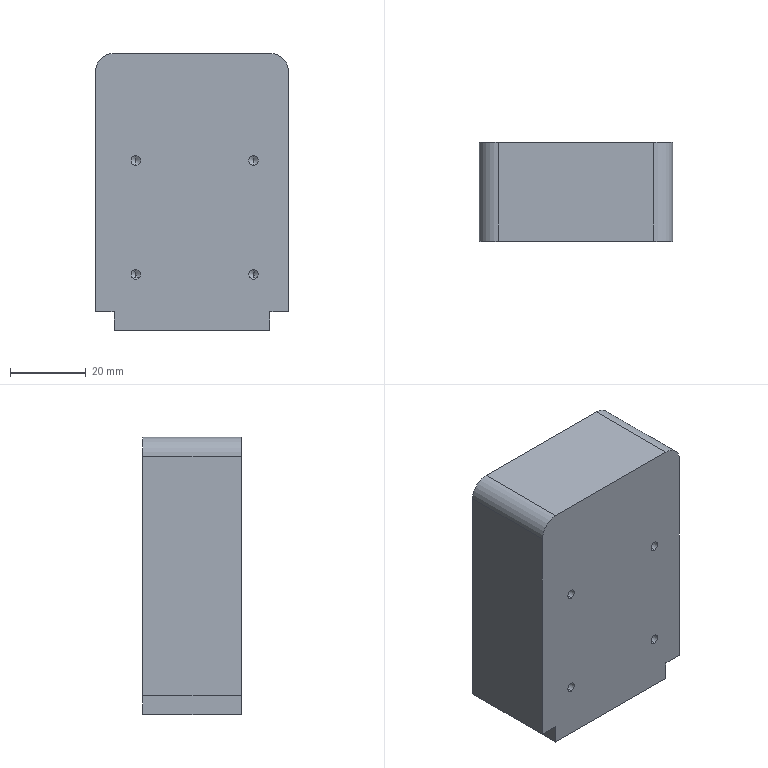Part | SolidWorks | features Extrusion 1, Fillet 1, HoleWzd 1, ICE 1 | 1 solid | 28 faces | box 51 x 26 x 73 mm | volume 95067 mm3 | cylinder 10 | plane 10 | cone 8 | commonest cylinder face diameters 2.5 x8 10 x2
STEP:
#1=CARTESIAN_POINT('',(-14.8,7.5,9.55));
#2=VERTEX_POINT('',#1);
#3=CARTESIAN_POINT('',(-14.8,7.5,7.05));
#4=VERTEX_POINT('',#3);
#5=CARTESIAN_POINT('',(-14.8,7.5,8.3));
#6=DIRECTION('',(0.,-1.,0.));
#7=DIRECTION('',(0.,0.,-1.));
#8=AXIS2_PLACEMENT_3D('',#5,#6,#7);
#9=CIRCLE('',#8,1.25);
#10=EDGE_CURVE('',#2,#4,#9,.T.);
#11=ORIENTED_EDGE('',*,*,#10,.F.);
#12=CARTESIAN_POINT('',(-14.8,0.,9.55));
#13=VERTEX_POINT('',#12);
#14=CARTESIAN_POINT('',(-14.8,0.,9.55));
#15=DIRECTION('',(0.,-1.,0.));
#16=VECTOR('',#15,1000.);
#17=LINE('',#14,#16);
#18=EDGE_CURVE('',#2,#13,#17,.T.);
#19=ORIENTED_EDGE('',*,*,#18,.T.);
#20=CARTESIAN_POINT('',(-14.8,0.,7.05));
#21=VERTEX_POINT('',#20);
#22=CARTESIAN_POINT('',(-14.8,0.,8.3));
#23=DIRECTION('',(0.,-1.,0.));
#24=DIRECTION('',(0.,0.,-1.));
#25=AXIS2_PLACEMENT_3D('',#22,#23,#24);
#26=CIRCLE('',#25,1.25);
#27=EDGE_CURVE('',#13,#21,#26,.T.);
#28=ORIENTED_EDGE('',*,*,#27,.T.);
#29=CARTESIAN_POINT('',(-14.8,0.,7.05));
#30=DIRECTION('',(0.,-1.,0.));
#31=VECTOR('',#30,1000.);
#32=LINE('',#29,#31);
#33=EDGE_CURVE('',#4,#21,#32,.T.);
#34=ORIENTED_EDGE('',*,*,#33,.F.);
#35=EDGE_LOOP('',(#11,#19,#28,#34));
#36=FACE_OUTER_BOUND('',#35,.T.);
#37=CARTESIAN_POINT('',(-14.8,0.,8.3));
#38=DIRECTION('',(0.,-1.,0.));
#39=DIRECTION('',(0.,0.,-1.));
#40=AXIS2_PLACEMENT_3D('',#37,#38,#39);
#41=CYLINDRICAL_SURFACE('',#40,1.25);
#42=ADVANCED_FACE('',(#36),#41,.F.);
#43=CARTESIAN_POINT('',(-14.8,8.251,8.3));
#44=VERTEX_POINT('',#43);
#45=CARTESIAN_POINT('',(-14.8,7.5,7.05));
#46=DIRECTION('',(0.,-0.515,-0.8572));
#47=VECTOR('',#46,1000.);
#48=LINE('',#45,#47);
#49=EDGE_CURVE('',#44,#4,#48,.T.);
#50=ORIENTED_EDGE('',*,*,#49,.F.);
#51=CARTESIAN_POINT('',(-14.8,7.5,9.55));
#52=DIRECTION('',(0.,-0.515,0.8572));
#53=VECTOR('',#52,1000.);
#54=LINE('',#51,#53);
#55=EDGE_CURVE('',#44,#2,#54,.T.);
#56=ORIENTED_EDGE('',*,*,#55,.T.);
#57=ORIENTED_EDGE('',*,*,#10,.T.);
#58=EDGE_LOOP('',(#50,#56,#57));
#59=FACE_OUTER_BOUND('',#58,.T.);
#60=CARTESIAN_POINT('',(-14.8,7.5,8.3));
#61=DIRECTION('',(0.,-1.,0.));
#62=DIRECTION('',(0.,0.,-1.));
#63=AXIS2_PLACEMENT_3D('',#60,#61,#62);
#64=CONICAL_SURFACE('',#63,1.25,1.03);
#65=ADVANCED_FACE('',(#59),#64,.F.);
#66=CARTESIAN_POINT('',(16.2,7.5,9.55));
#67=VERTEX_POINT('',#66);
#68=CARTESIAN_POINT('',(16.2,7.5,7.05));
#69=VERTEX_POINT('',#68);
#70=CARTESIAN_POINT('',(16.2,7.5,8.3));
#71=DIRECTION('',(0.,-1.,0.));
#72=DIRECTION('',(0.,0.,-1.));
#73=AXIS2_PLACEMENT_3D('',#70,#71,#72);
#74=CIRCLE('',#73,1.25);
#75=EDGE_CURVE('',#67,#69,#74,.T.);
#76=ORIENTED_EDGE('',*,*,#75,.F.);
#77=CARTESIAN_POINT('',(16.2,0.,9.55));
#78=VERTEX_POINT('',#77);
#79=CARTESIAN_POINT('',(16.2,0.,9.55));
#80=DIRECTION('',(0.,-1.,0.));
#81=VECTOR('',#80,1000.);
#82=LINE('',#79,#81);
#83=EDGE_CURVE('',#67,#78,#82,.T.);
#84=ORIENTED_EDGE('',*,*,#83,.T.);
#85=CARTESIAN_POINT('',(16.2,0.,7.05));
#86=VERTEX_POINT('',#85);
#87=CARTESIAN_POINT('',(16.2,0.,8.3));
#88=DIRECTION('',(0.,-1.,0.));
#89=DIRECTION('',(0.,0.,-1.));
#90=AXIS2_PLACEMENT_3D('',#87,#88,#89);
#91=CIRCLE('',#90,1.25);
#92=EDGE_CURVE('',#78,#86,#91,.T.);
#93=ORIENTED_EDGE('',*,*,#92,.T.);
#94=CARTESIAN_POINT('',(16.2,0.,7.05));
#95=DIRECTION('',(0.,-1.,0.));
#96=VECTOR('',#95,1000.);
#97=LINE('',#94,#96);
#98=EDGE_CURVE('',#69,#86,#97,.T.);
#99=ORIENTED_EDGE('',*,*,#98,.F.);
#100=EDGE_LOOP('',(#76,#84,#93,#99));
#101=FACE_OUTER_BOUND('',#100,.T.);
#102=CARTESIAN_POINT('',(16.2,0.,8.3));
#103=DIRECTION('',(0.,-1.,0.));
#104=DIRECTION('',(0.,0.,-1.));
#105=AXIS2_PLACEMENT_3D('',#102,#103,#104);
#106=CYLINDRICAL_SURFACE('',#105,1.25);
#107=ADVANCED_FACE('',(#101),#106,.F.);
#108=CARTESIAN_POINT('',(16.2,8.251,8.3));
#109=VERTEX_POINT('',#108);
#110=CARTESIAN_POINT('',(16.2,7.5,7.05));
#111=DIRECTION('',(0.,-0.515,-0.8572));
#112=VECTOR('',#111,1000.);
#113=LINE('',#110,#112);
#114=EDGE_CURVE('',#109,#69,#113,.T.);
#115=ORIENTED_EDGE('',*,*,#114,.F.);
#116=CARTESIAN_POINT('',(16.2,7.5,9.55));
#117=DIRECTION('',(0.,-0.515,0.8572));
#118=VECTOR('',#117,1000.);
#119=LINE('',#116,#118);
#120=EDGE_CURVE('',#109,#67,#119,.T.);
#121=ORIENTED_EDGE('',*,*,#120,.T.);
#122=ORIENTED_EDGE('',*,*,#75,.T.);
#123=EDGE_LOOP('',(#115,#121,#122));
#124=FACE_OUTER_BOUND('',#123,.T.);
#125=CARTESIAN_POINT('',(16.2,7.5,8.3));
#126=DIRECTION('',(0.,-1.,0.));
#127=DIRECTION('',(0.,0.,-1.));
#128=AXIS2_PLACEMENT_3D('',#125,#126,#127);
#129=CONICAL_SURFACE('',#128,1.25,1.03);
#130=ADVANCED_FACE('',(#124),#129,.F.);
#131=CARTESIAN_POINT('',(-14.8,7.5,-20.45));
#132=VERTEX_POINT('',#131);
#133=CARTESIAN_POINT('',(-14.8,7.5,-22.95));
#134=VERTEX_POINT('',#133);
#135=CARTESIAN_POINT('',(-14.8,7.5,-21.7));
#136=DIRECTION('',(0.,-1.,0.));
#137=DIRECTION('',(0.,0.,-1.));
#138=AXIS2_PLACEMENT_3D('',#135,#136,#137);
#139=CIRCLE('',#138,1.25);
#140=EDGE_CURVE('',#132,#134,#139,.T.);
#141=ORIENTED_EDGE('',*,*,#140,.F.);
#142=CARTESIAN_POINT('',(-14.8,0.,-20.45));
#143=VERTEX_POINT('',#142);
#144=CARTESIAN_POINT('',(-14.8,0.,-20.45));
#145=DIRECTION('',(0.,-1.,0.));
#146=VECTOR('',#145,1000.);
#147=LINE('',#144,#146);
#148=EDGE_CURVE('',#132,#143,#147,.T.);
#149=ORIENTED_EDGE('',*,*,#148,.T.);
#150=CARTESIAN_POINT('',(-14.8,0.,-22.95));
#151=VERTEX_POINT('',#150);
#152=CARTESIAN_POINT('',(-14.8,0.,-21.7));
#153=DIRECTION('',(0.,-1.,0.));
#154=DIRECTION('',(0.,0.,-1.));
#155=AXIS2_PLACEMENT_3D('',#152,#153,#154);
#156=CIRCLE('',#155,1.25);
#157=EDGE_CURVE('',#143,#151,#156,.T.);
#158=ORIENTED_EDGE('',*,*,#157,.T.);
#159=CARTESIAN_POINT('',(-14.8,0.,-22.95));
#160=DIRECTION('',(0.,-1.,0.));
#161=VECTOR('',#160,1000.);
#162=LINE('',#159,#161);
#163=EDGE_CURVE('',#134,#151,#162,.T.);
#164=ORIENTED_EDGE('',*,*,#163,.F.);
#165=EDGE_LOOP('',(#141,#149,#158,#164));
#166=FACE_OUTER_BOUND('',#165,.T.);
#167=CARTESIAN_POINT('',(-14.8,0.,-21.7));
#168=DIRECTION('',(0.,-1.,0.));
#169=DIRECTION('',(0.,0.,-1.));
#170=AXIS2_PLACEMENT_3D('',#167,#168,#169);
#171=CYLINDRICAL_SURFACE('',#170,1.25);
#172=ADVANCED_FACE('',(#166),#171,.F.);
#173=CARTESIAN_POINT('',(-14.8,8.251,-21.7));
#174=VERTEX_POINT('',#173);
#175=CARTESIAN_POINT('',(-14.8,7.5,-22.95));
#176=DIRECTION('',(0.,-0.515,-0.8572));
#177=VECTOR('',#176,1000.);
#178=LINE('',#175,#177);
#179=EDGE_CURVE('',#174,#134,#178,.T.);
#180=ORIENTED_EDGE('',*,*,#179,.F.);
#181=CARTESIAN_POINT('',(-14.8,7.5,-20.45));
#182=DIRECTION('',(0.,-0.515,0.8572));
#183=VECTOR('',#182,1000.);
#184=LINE('',#181,#183);
#185=EDGE_CURVE('',#174,#132,#184,.T.);
#186=ORIENTED_EDGE('',*,*,#185,.T.);
#187=ORIENTED_EDGE('',*,*,#140,.T.);
#188=EDGE_LOOP('',(#180,#186,#187));
#189=FACE_OUTER_BOUND('',#188,.T.);
#190=CARTESIAN_POINT('',(-14.8,7.5,-21.7));
#191=DIRECTION('',(0.,-1.,0.));
#192=DIRECTION('',(0.,0.,-1.));
#193=AXIS2_PLACEMENT_3D('',#190,#191,#192);
#194=CONICAL_SURFACE('',#193,1.25,1.03);
#195=ADVANCED_FACE('',(#189),#194,.F.);
#196=CARTESIAN_POINT('',(16.2,7.5,-20.45));
#197=VERTEX_POINT('',#196);
#198=CARTESIAN_POINT('',(16.2,7.5,-22.95));
#199=VERTEX_POINT('',#198);
#200=CARTESIAN_POINT('',(16.2,7.5,-21.7));
#201=DIRECTION('',(0.,-1.,0.));
#202=DIRECTION('',(0.,0.,-1.));
#203=AXIS2_PLACEMENT_3D('',#200,#201,#202);
#204=CIRCLE('',#203,1.25);
#205=EDGE_CURVE('',#197,#199,#204,.T.);
#206=ORIENTED_EDGE('',*,*,#205,.F.);
#207=CARTESIAN_POINT('',(16.2,0.,-20.45));
#208=VERTEX_POINT('',#207);
#209=CARTESIAN_POINT('',(16.2,0.,-20.45));
#210=DIRECTION('',(0.,-1.,0.));
#211=VECTOR('',#210,1000.);
#212=LINE('',#209,#211);
#213=EDGE_CURVE('',#197,#208,#212,.T.);
#214=ORIENTED_EDGE('',*,*,#213,.T.);
#215=CARTESIAN_POINT('',(16.2,0.,-22.95));
#216=VERTEX_POINT('',#215);
#217=CARTESIAN_POINT('',(16.2,0.,-21.7));
#218=DIRECTION('',(0.,-1.,0.));
#219=DIRECTION('',(0.,0.,-1.));
#220=AXIS2_PLACEMENT_3D('',#217,#218,#219);
#221=CIRCLE('',#220,1.25);
#222=EDGE_CURVE('',#208,#216,#221,.T.);
#223=ORIENTED_EDGE('',*,*,#222,.T.);
#224=CARTESIAN_POINT('',(16.2,0.,-22.95));
#225=DIRECTION('',(0.,-1.,0.));
#226=VECTOR('',#225,1000.);
#227=LINE('',#224,#226);
#228=EDGE_CURVE('',#199,#216,#227,.T.);
#229=ORIENTED_EDGE('',*,*,#228,.F.);
#230=EDGE_LOOP('',(#206,#214,#223,#229));
#231=FACE_OUTER_BOUND('',#230,.T.);
#232=CARTESIAN_POINT('',(16.2,0.,-21.7));
#233=DIRECTION('',(0.,-1.,0.));
#234=DIRECTION('',(0.,0.,-1.));
#235=AXIS2_PLACEMENT_3D('',#232,#233,#234);
#236=CYLINDRICAL_SURFACE('',#235,1.25);
#237=ADVANCED_FACE('',(#231),#236,.F.);
#238=CARTESIAN_POINT('',(16.2,8.251,-21.7));
#239=VERTEX_POINT('',#238);
#240=CARTESIAN_POINT('',(16.2,7.5,-22.95));
#241=DIRECTION('',(0.,-0.515,-0.8572));
#242=VECTOR('',#241,1000.);
#243=LINE('',#240,#242);
#244=EDGE_CURVE('',#239,#199,#243,.T.);
#245=ORIENTED_EDGE('',*,*,#244,.F.);
#246=CARTESIAN_POINT('',(16.2,7.5,-20.45));
#247=DIRECTION('',(0.,-0.515,0.8572));
#248=VECTOR('',#247,1000.);
#249=LINE('',#246,#248);
#250=EDGE_CURVE('',#239,#197,#249,.T.);
#251=ORIENTED_EDGE('',*,*,#250,.T.);
#252=ORIENTED_EDGE('',*,*,#205,.T.);
#253=EDGE_LOOP('',(#245,#251,#252));
#254=FACE_OUTER_BOUND('',#253,.T.);
#255=CARTESIAN_POINT('',(16.2,7.5,-21.7));
#256=DIRECTION('',(0.,-1.,0.));
#257=DIRECTION('',(0.,0.,-1.));
#258=AXIS2_PLACEMENT_3D('',#255,#256,#257);
#259=CONICAL_SURFACE('',#258,1.25,1.03);
#260=ADVANCED_FACE('',(#254),#259,.F.);
#261=CARTESIAN_POINT('',(25.5,26.,31.5));
#262=VERTEX_POINT('',#261);
#263=CARTESIAN_POINT('',(25.5,26.,-31.5));
#264=VERTEX_POINT('',#263);
#265=CARTESIAN_POINT('',(25.5,26.,-36.5));
#266=DIRECTION('',(0.,0.,-1.));
#267=VECTOR('',#266,1000.);
#268=LINE('',#265,#267);
#269=EDGE_CURVE('',#262,#264,#268,.T.);
#270=ORIENTED_EDGE('',*,*,#269,.F.);
#271=CARTESIAN_POINT('',(25.5,0.,31.5));
#272=VERTEX_POINT('',#271);
#273=CARTESIAN_POINT('',(25.5,26.,31.5));
#274=DIRECTION('',(0.,-1.,0.));
#275=VECTOR('',#274,1000.);
#276=LINE('',#273,#275);
#277=EDGE_CURVE('',#262,#272,#276,.T.);
#278=ORIENTED_EDGE('',*,*,#277,.T.);
#279=CARTESIAN_POINT('',(25.5,0.,-31.5));
#280=VERTEX_POINT('',#279);
#281=CARTESIAN_POINT('',(25.5,0.,-36.5));
#282=DIRECTION('',(0.,0.,-1.));
#283=VECTOR('',#282,1000.);
#284=LINE('',#281,#283);
#285=EDGE_CURVE('',#272,#280,#284,.T.);
#286=ORIENTED_EDGE('',*,*,#285,.T.);
#287=CARTESIAN_POINT('',(25.5,26.,-31.5));
#288=DIRECTION('',(0.,1.,0.));
#289=VECTOR('',#288,1000.);
#290=LINE('',#287,#289);
#291=EDGE_CURVE('',#280,#264,#290,.T.);
#292=ORIENTED_EDGE('',*,*,#291,.T.);
#293=EDGE_LOOP('',(#270,#278,#286,#292));
#294=FACE_OUTER_BOUND('',#293,.T.);
#295=CARTESIAN_POINT('',(25.5,26.,-36.5));
#296=DIRECTION('',(-1.,0.,0.));
#297=DIRECTION('',(0.,0.,1.));
#298=AXIS2_PLACEMENT_3D('',#295,#296,#297);
#299=PLANE('',#298);
#300=ADVANCED_FACE('',(#294),#299,.F.);
#301=CARTESIAN_POINT('',(20.5,26.,-36.5));
#302=VERTEX_POINT('',#301);
#303=CARTESIAN_POINT('',(-20.5,26.,-36.5));
#304=VERTEX_POINT('',#303);
#305=CARTESIAN_POINT('',(-25.5,26.,-36.5));
#306=DIRECTION('',(-1.,0.,0.));
#307=VECTOR('',#306,1000.);
#308=LINE('',#305,#307);
#309=EDGE_CURVE('',#302,#304,#308,.T.);
#310=ORIENTED_EDGE('',*,*,#309,.F.);
#311=CARTESIAN_POINT('',(20.5,0.,-36.5));
#312=VERTEX_POINT('',#311);
#313=CARTESIAN_POINT('',(20.5,26.,-36.5));
#314=DIRECTION('',(0.,-1.,0.));
#315=VECTOR('',#314,1000.);
#316=LINE('',#313,#315);
#317=EDGE_CURVE('',#302,#312,#316,.T.);
#318=ORIENTED_EDGE('',*,*,#317,.T.);
#319=CARTESIAN_POINT('',(-20.5,0.,-36.5));
#320=VERTEX_POINT('',#319);
#321=CARTESIAN_POINT('',(-25.5,0.,-36.5));
#322=DIRECTION('',(-1.,0.,0.));
#323=VECTOR('',#322,1000.);
#324=LINE('',#321,#323);
#325=EDGE_CURVE('',#312,#320,#324,.T.);
#326=ORIENTED_EDGE('',*,*,#325,.T.);
#327=CARTESIAN_POINT('',(-20.5,26.,-36.5));
#328=DIRECTION('',(0.,1.,0.));
#329=VECTOR('',#328,1000.);
#330=LINE('',#327,#329);
#331=EDGE_CURVE('',#320,#304,#330,.T.);
#332=ORIENTED_EDGE('',*,*,#331,.T.);
#333=EDGE_LOOP('',(#310,#318,#326,#332));
#334=FACE_OUTER_BOUND('',#333,.T.);
#335=CARTESIAN_POINT('',(-25.5,26.,-36.5));
#336=DIRECTION('',(0.,0.,1.));
#337=DIRECTION('',(1.,0.,0.));
#338=AXIS2_PLACEMENT_3D('',#335,#336,#337);
#339=PLANE('',#338);
#340=ADVANCED_FACE('',(#334),#339,.F.);
#341=CARTESIAN_POINT('',(-25.5,26.,-31.5));
#342=VERTEX_POINT('',#341);
#343=CARTESIAN_POINT('',(-25.5,26.,31.5));
#344=VERTEX_POINT('',#343);
#345=CARTESIAN_POINT('',(-25.5,26.,-36.5));
#346=DIRECTION('',(0.,0.,1.));
#347=VECTOR('',#346,1000.);
#348=LINE('',#345,#347);
#349=EDGE_CURVE('',#342,#344,#348,.T.);
#350=ORIENTED_EDGE('',*,*,#349,.F.);
#351=CARTESIAN_POINT('',(-25.5,0.,-31.5));
#352=VERTEX_POINT('',#351);
#353=CARTESIAN_POINT('',(-25.5,26.,-31.5));
#354=DIRECTION('',(0.,-1.,0.));
#355=VECTOR('',#354,1000.);
#356=LINE('',#353,#355);
#357=EDGE_CURVE('',#342,#352,#356,.T.);
#358=ORIENTED_EDGE('',*,*,#357,.T.);
#359=CARTESIAN_POINT('',(-25.5,0.,31.5));
#360=VERTEX_POINT('',#359);
#361=CARTESIAN_POINT('',(-25.5,0.,-36.5));
#362=DIRECTION('',(0.,0.,1.));
#363=VECTOR('',#362,1000.);
#364=LINE('',#361,#363);
#365=EDGE_CURVE('',#352,#360,#364,.T.);
#366=ORIENTED_EDGE('',*,*,#365,.T.);
#367=CARTESIAN_POINT('',(-25.5,26.,31.5));
#368=DIRECTION('',(0.,1.,0.));
#369=VECTOR('',#368,1000.);
#370=LINE('',#367,#369);
#371=EDGE_CURVE('',#360,#344,#370,.T.);
#372=ORIENTED_EDGE('',*,*,#371,.T.);
#373=EDGE_LOOP('',(#350,#358,#366,#372));
#374=FACE_OUTER_BOUND('',#373,.T.);
#375=CARTESIAN_POINT('',(-25.5,26.,-36.5));
#376=DIRECTION('',(1.,0.,0.));
#377=DIRECTION('',(0.,0.,-1.));
#378=AXIS2_PLACEMENT_3D('',#375,#376,#377);
#379=PLANE('',#378);
#380=ADVANCED_FACE('',(#374),#379,.F.);
#381=CARTESIAN_POINT('',(-20.5,0.,36.5));
#382=VERTEX_POINT('',#381);
#383=CARTESIAN_POINT('',(20.5,0.,36.5));
#384=VERTEX_POINT('',#383);
#385=CARTESIAN_POINT('',(-25.5,0.,36.5));
#386=DIRECTION('',(1.,0.,0.));
#387=VECTOR('',#386,1000.);
#388=LINE('',#385,#387);
#389=EDGE_CURVE('',#382,#384,#388,.T.);
#390=ORIENTED_EDGE('',*,*,#389,.T.);
#391=CARTESIAN_POINT('',(20.5,26.,36.5));
#392=VERTEX_POINT('',#391);
#393=CARTESIAN_POINT('',(20.5,26.,36.5));
#394=DIRECTION('',(0.,1.,0.));
#395=VECTOR('',#394,1000.);
#396=LINE('',#393,#395);
#397=EDGE_CURVE('',#384,#392,#396,.T.);
#398=ORIENTED_EDGE('',*,*,#397,.T.);
#399=CARTESIAN_POINT('',(-20.5,26.,36.5));
#400=VERTEX_POINT('',#399);
#401=CARTESIAN_POINT('',(-25.5,26.,36.5));
#402=DIRECTION('',(1.,0.,0.));
#403=VECTOR('',#402,1000.);
#404=LINE('',#401,#403);
#405=EDGE_CURVE('',#400,#392,#404,.T.);
#406=ORIENTED_EDGE('',*,*,#405,.F.);
#407=CARTESIAN_POINT('',(-20.5,26.,36.5));
#408=DIRECTION('',(0.,-1.,0.));
#409=VECTOR('',#408,1000.);
#410=LINE('',#407,#409);
#411=EDGE_CURVE('',#400,#382,#410,.T.);
#412=ORIENTED_EDGE('',*,*,#411,.T.);
#413=EDGE_LOOP('',(#390,#398,#406,#412));
#414=FACE_OUTER_BOUND('',#413,.T.);
#415=CARTESIAN_POINT('',(-25.5,26.,36.5));
#416=DIRECTION('',(0.,0.,-1.));
#417=DIRECTION('',(-1.,0.,0.));
#418=AXIS2_PLACEMENT_3D('',#415,#416,#417);
#419=PLANE('',#418);
#420=ADVANCED_FACE('',(#414),#419,.F.);
#421=CARTESIAN_POINT('',(20.5,26.,-31.5));
#422=VERTEX_POINT('',#421);
#423=CARTESIAN_POINT('',(20.5,26.,0.));
#424=DIRECTION('',(0.,0.,1.));
#425=VECTOR('',#424,1000.);
#426=LINE('',#423,#425);
#427=EDGE_CURVE('',#302,#422,#426,.T.);
#428=ORIENTED_EDGE('',*,*,#427,.F.);
#429=ORIENTED_EDGE('',*,*,#309,.T.);
#430=CARTESIAN_POINT('',(-20.5,26.,-31.5));
#431=VERTEX_POINT('',#430);
#432=CARTESIAN_POINT('',(-20.5,26.,0.));
#433=DIRECTION('',(0.,0.,-1.));
#434=VECTOR('',#433,1000.);
#435=LINE('',#432,#434);
#436=EDGE_CURVE('',#431,#304,#435,.T.);
#437=ORIENTED_EDGE('',*,*,#436,.F.);
#438=CARTESIAN_POINT('',(0.,26.,-31.5));
#439=DIRECTION('',(1.,0.,0.));
#440=VECTOR('',#439,1000.);
#441=LINE('',#438,#440);
#442=EDGE_CURVE('',#342,#431,#441,.T.);
#443=ORIENTED_EDGE('',*,*,#442,.F.);
#444=ORIENTED_EDGE('',*,*,#349,.T.);
#445=CARTESIAN_POINT('',(-20.5,26.,31.5));
#446=DIRECTION('',(0.,1.,0.));
#447=DIRECTION('',(0.,0.,1.));
#448=AXIS2_PLACEMENT_3D('',#445,#446,#447);
#449=CIRCLE('',#448,5.);
#450=EDGE_CURVE('',#344,#400,#449,.T.);
#451=ORIENTED_EDGE('',*,*,#450,.T.);
#452=ORIENTED_EDGE('',*,*,#405,.T.);
#453=CARTESIAN_POINT('',(20.5,26.,31.5));
#454=DIRECTION('',(0.,1.,0.));
#455=DIRECTION('',(0.,0.,1.));
#456=AXIS2_PLACEMENT_3D('',#453,#454,#455);
#457=CIRCLE('',#456,5.);
#458=EDGE_CURVE('',#392,#262,#457,.T.);
#459=ORIENTED_EDGE('',*,*,#458,.T.);
#460=ORIENTED_EDGE('',*,*,#269,.T.);
#461=CARTESIAN_POINT('',(0.,26.,-31.5));
#462=DIRECTION('',(1.,0.,0.));
#463=VECTOR('',#462,1000.);
#464=LINE('',#461,#463);
#465=EDGE_CURVE('',#422,#264,#464,.T.);
#466=ORIENTED_EDGE('',*,*,#465,.F.);
#467=EDGE_LOOP('',(#428,#429,#437,#443,#444,#451,#452,#459,#460,#466));
#468=FACE_OUTER_BOUND('',#467,.T.);
#469=CARTESIAN_POINT('',(0.,26.,0.));
#470=DIRECTION('',(0.,1.,0.));
#471=DIRECTION('',(0.,0.,1.));
#472=AXIS2_PLACEMENT_3D('',#469,#470,#471);
#473=PLANE('',#472);
#474=ADVANCED_FACE('',(#468),#473,.T.);
#475=CARTESIAN_POINT('',(-14.8,0.,8.3));
#476=DIRECTION('',(0.,-1.,0.));
#477=DIRECTION('',(0.,0.,-1.));
#478=AXIS2_PLACEMENT_3D('',#475,#476,#477);
#479=CIRCLE('',#478,1.25);
#480=EDGE_CURVE('',#21,#13,#479,.T.);
#481=ORIENTED_EDGE('',*,*,#480,.F.);
#482=ORIENTED_EDGE('',*,*,#27,.F.);
#483=EDGE_LOOP('',(#481,#482));
#484=FACE_BOUND('',#483,.T.);
#485=CARTESIAN_POINT('',(16.2,0.,8.3));
#486=DIRECTION('',(0.,-1.,0.));
#487=DIRECTION('',(0.,0.,-1.));
#488=AXIS2_PLACEMENT_3D('',#485,#486,#487);
#489=CIRCLE('',#488,1.25);
#490=EDGE_CURVE('',#86,#78,#489,.T.);
#491=ORIENTED_EDGE('',*,*,#490,.F.);
#492=ORIENTED_EDGE('',*,*,#92,.F.);
#493=EDGE_LOOP('',(#491,#492));
#494=FACE_BOUND('',#493,.T.);
#495=CARTESIAN_POINT('',(-14.8,0.,-21.7));
#496=DIRECTION('',(0.,-1.,0.));
#497=DIRECTION('',(0.,0.,-1.));
#498=AXIS2_PLACEMENT_3D('',#495,#496,#497);
#499=CIRCLE('',#498,1.25);
#500=EDGE_CURVE('',#151,#143,#499,.T.);
#501=ORIENTED_EDGE('',*,*,#500,.F.);
#502=ORIENTED_EDGE('',*,*,#157,.F.);
#503=EDGE_LOOP('',(#501,#502));
#504=FACE_BOUND('',#503,.T.);
#505=CARTESIAN_POINT('',(16.2,0.,-21.7));
#506=DIRECTION('',(0.,-1.,0.));
#507=DIRECTION('',(0.,0.,-1.));
#508=AXIS2_PLACEMENT_3D('',#505,#506,#507);
#509=CIRCLE('',#508,1.25);
#510=EDGE_CURVE('',#216,#208,#509,.T.);
#511=ORIENTED_EDGE('',*,*,#510,.F.);
#512=ORIENTED_EDGE('',*,*,#222,.F.);
#513=EDGE_LOOP('',(#511,#512));
#514=FACE_BOUND('',#513,.T.);
#515=ORIENTED_EDGE('',*,*,#325,.F.);
#516=CARTESIAN_POINT('',(20.5,0.,-31.5));
#517=VERTEX_POINT('',#516);
#518=CARTESIAN_POINT('',(20.5,0.,-36.5));
#519=DIRECTION('',(0.,0.,-1.));
#520=VECTOR('',#519,1000.);
#521=LINE('',#518,#520);
#522=EDGE_CURVE('',#517,#312,#521,.T.);
#523=ORIENTED_EDGE('',*,*,#522,.F.);
#524=CARTESIAN_POINT('',(25.5,0.,-31.5));
#525=DIRECTION('',(-1.,0.,0.));
#526=VECTOR('',#525,1000.);
#527=LINE('',#524,#526);
#528=EDGE_CURVE('',#280,#517,#527,.T.);
#529=ORIENTED_EDGE('',*,*,#528,.F.);
#530=ORIENTED_EDGE('',*,*,#285,.F.);
#531=CARTESIAN_POINT('',(20.5,0.,31.5));
#532=DIRECTION('',(0.,-1.,0.));
#533=DIRECTION('',(0.,0.,1.));
#534=AXIS2_PLACEMENT_3D('',#531,#532,#533);
#535=CIRCLE('',#534,5.);
#536=EDGE_CURVE('',#272,#384,#535,.T.);
#537=ORIENTED_EDGE('',*,*,#536,.T.);
#538=ORIENTED_EDGE('',*,*,#389,.F.);
#539=CARTESIAN_POINT('',(-20.5,0.,31.5));
#540=DIRECTION('',(0.,-1.,0.));
#541=DIRECTION('',(0.,0.,1.));
#542=AXIS2_PLACEMENT_3D('',#539,#540,#541);
#543=CIRCLE('',#542,5.);
#544=EDGE_CURVE('',#382,#360,#543,.T.);
#545=ORIENTED_EDGE('',*,*,#544,.T.);
#546=ORIENTED_EDGE('',*,*,#365,.F.);
#547=CARTESIAN_POINT('',(-20.5,0.,-31.5));
#548=VERTEX_POINT('',#547);
#549=CARTESIAN_POINT('',(-25.5,0.,-31.5));
#550=DIRECTION('',(-1.,0.,0.));
#551=VECTOR('',#550,1000.);
#552=LINE('',#549,#551);
#553=EDGE_CURVE('',#548,#352,#552,.T.);
#554=ORIENTED_EDGE('',*,*,#553,.F.);
#555=CARTESIAN_POINT('',(-20.5,0.,-36.5));
#556=DIRECTION('',(0.,0.,1.));
#557=VECTOR('',#556,1000.);
#558=LINE('',#555,#557);
#559=EDGE_CURVE('',#320,#548,#558,.T.);
#560=ORIENTED_EDGE('',*,*,#559,.F.);
#561=EDGE_LOOP('',(#515,#523,#529,#530,#537,#538,#545,#546,#554,#560));
#562=FACE_OUTER_BOUND('',#561,.T.);
#563=CARTESIAN_POINT('',(0.,0.,0.));
#564=DIRECTION('',(0.,1.,0.));
#565=DIRECTION('',(0.,0.,1.));
#566=AXIS2_PLACEMENT_3D('',#563,#564,#565);
#567=PLANE('',#566);
#568=ADVANCED_FACE('',(#484,#494,#504,#514,#562),#567,.F.);
#569=ORIENTED_EDGE('',*,*,#458,.F.);
#570=ORIENTED_EDGE('',*,*,#397,.F.);
#571=ORIENTED_EDGE('',*,*,#536,.F.);
#572=ORIENTED_EDGE('',*,*,#277,.F.);
#573=EDGE_LOOP('',(#569,#570,#571,#572));
#574=FACE_OUTER_BOUND('',#573,.T.);
#575=CARTESIAN_POINT('',(20.5,26.,31.5));
#576=DIRECTION('',(0.,-1.,0.));
#577=DIRECTION('',(0.,0.,-1.));
#578=AXIS2_PLACEMENT_3D('',#575,#576,#577);
#579=CYLINDRICAL_SURFACE('',#578,5.);
#580=ADVANCED_FACE('',(#574),#579,.T.);
#581=ORIENTED_EDGE('',*,*,#450,.F.);
#582=ORIENTED_EDGE('',*,*,#371,.F.);
#583=ORIENTED_EDGE('',*,*,#544,.F.);
#584=ORIENTED_EDGE('',*,*,#411,.F.);
#585=EDGE_LOOP('',(#581,#582,#583,#584));
#586=FACE_OUTER_BOUND('',#585,.T.);
#587=CARTESIAN_POINT('',(-20.5,26.,31.5));
#588=DIRECTION('',(0.,-1.,0.));
#589=DIRECTION('',(0.,0.,-1.));
#590=AXIS2_PLACEMENT_3D('',#587,#588,#589);
#591=CYLINDRICAL_SURFACE('',#590,5.);
#592=ADVANCED_FACE('',(#586),#591,.T.);
#593=ORIENTED_EDGE('',*,*,#442,.T.);
#594=CARTESIAN_POINT('',(-20.5,30.,-31.5));
#595=DIRECTION('',(0.,-1.,0.));
#596=VECTOR('',#595,1000.);
#597=LINE('',#594,#596);
#598=EDGE_CURVE('',#431,#548,#597,.T.);
#599=ORIENTED_EDGE('',*,*,#598,.T.);
#600=ORIENTED_EDGE('',*,*,#553,.T.);
#601=ORIENTED_EDGE('',*,*,#357,.F.);
#602=EDGE_LOOP('',(#593,#599,#600,#601));
#603=FACE_OUTER_BOUND('',#602,.T.);
#604=CARTESIAN_POINT('',(-25.5,30.,-31.5));
#605=DIRECTION('',(0.,0.,1.));
#606=DIRECTION('',(1.,0.,0.));
#607=AXIS2_PLACEMENT_3D('',#604,#605,#606);
#608=PLANE('',#607);
#609=ADVANCED_FACE('',(#603),#608,.F.);
#610=ORIENTED_EDGE('',*,*,#436,.T.);
#611=ORIENTED_EDGE('',*,*,#331,.F.);
#612=ORIENTED_EDGE('',*,*,#559,.T.);
#613=ORIENTED_EDGE('',*,*,#598,.F.);
#614=EDGE_LOOP('',(#610,#611,#612,#613));
#615=FACE_OUTER_BOUND('',#614,.T.);
#616=CARTESIAN_POINT('',(-20.5,30.,-36.5));
#617=DIRECTION('',(1.,0.,0.));
#618=DIRECTION('',(0.,0.,-1.));
#619=AXIS2_PLACEMENT_3D('',#616,#617,#618);
#620=PLANE('',#619);
#621=ADVANCED_FACE('',(#615),#620,.F.);
#622=ORIENTED_EDGE('',*,*,#427,.T.);
#623=CARTESIAN_POINT('',(20.5,30.,-31.5));
#624=DIRECTION('',(0.,-1.,0.));
#625=VECTOR('',#624,1000.);
#626=LINE('',#623,#625);
#627=EDGE_CURVE('',#422,#517,#626,.T.);
#628=ORIENTED_EDGE('',*,*,#627,.T.);
#629=ORIENTED_EDGE('',*,*,#522,.T.);
#630=ORIENTED_EDGE('',*,*,#317,.F.);
#631=EDGE_LOOP('',(#622,#628,#629,#630));
#632=FACE_OUTER_BOUND('',#631,.T.);
#633=CARTESIAN_POINT('',(20.5,30.,-36.5));
#634=DIRECTION('',(-1.,0.,0.));
#635=DIRECTION('',(0.,0.,1.));
#636=AXIS2_PLACEMENT_3D('',#633,#634,#635);
#637=PLANE('',#636);
#638=ADVANCED_FACE('',(#632),#637,.F.);
#639=ORIENTED_EDGE('',*,*,#465,.T.);
#640=ORIENTED_EDGE('',*,*,#291,.F.);
#641=ORIENTED_EDGE('',*,*,#528,.T.);
#642=ORIENTED_EDGE('',*,*,#627,.F.);
#643=EDGE_LOOP('',(#639,#640,#641,#642));
#644=FACE_OUTER_BOUND('',#643,.T.);
#645=CARTESIAN_POINT('',(25.5,30.,-31.5));
#646=DIRECTION('',(0.,0.,1.));
#647=DIRECTION('',(1.,0.,0.));
#648=AXIS2_PLACEMENT_3D('',#645,#646,#647);
#649=PLANE('',#648);
#650=ADVANCED_FACE('',(#644),#649,.F.);
#651=ORIENTED_EDGE('',*,*,#250,.F.);
#652=ORIENTED_EDGE('',*,*,#244,.T.);
#653=CARTESIAN_POINT('',(16.2,7.5,-21.7));
#654=DIRECTION('',(0.,-1.,0.));
#655=DIRECTION('',(0.,0.,-1.));
#656=AXIS2_PLACEMENT_3D('',#653,#654,#655);
#657=CIRCLE('',#656,1.25);
#658=EDGE_CURVE('',#199,#197,#657,.T.);
#659=ORIENTED_EDGE('',*,*,#658,.T.);
#660=EDGE_LOOP('',(#651,#652,#659));
#661=FACE_OUTER_BOUND('',#660,.T.);
#662=CARTESIAN_POINT('',(16.2,7.5,-21.7));
#663=DIRECTION('',(0.,-1.,0.));
#664=DIRECTION('',(0.,0.,-1.));
#665=AXIS2_PLACEMENT_3D('',#662,#663,#664);
#666=CONICAL_SURFACE('',#665,1.25,1.03);
#667=ADVANCED_FACE('',(#661),#666,.F.);
#668=ORIENTED_EDGE('',*,*,#213,.F.);
#669=ORIENTED_EDGE('',*,*,#658,.F.);
#670=ORIENTED_EDGE('',*,*,#228,.T.);
#671=ORIENTED_EDGE('',*,*,#510,.T.);
#672=EDGE_LOOP('',(#668,#669,#670,#671));
#673=FACE_OUTER_BOUND('',#672,.T.);
#674=CARTESIAN_POINT('',(16.2,0.,-21.7));
#675=DIRECTION('',(0.,-1.,0.));
#676=DIRECTION('',(0.,0.,-1.));
#677=AXIS2_PLACEMENT_3D('',#674,#675,#676);
#678=CYLINDRICAL_SURFACE('',#677,1.25);
#679=ADVANCED_FACE('',(#673),#678,.F.);
#680=ORIENTED_EDGE('',*,*,#185,.F.);
#681=ORIENTED_EDGE('',*,*,#179,.T.);
#682=CARTESIAN_POINT('',(-14.8,7.5,-21.7));
#683=DIRECTION('',(0.,-1.,0.));
#684=DIRECTION('',(0.,0.,-1.));
#685=AXIS2_PLACEMENT_3D('',#682,#683,#684);
#686=CIRCLE('',#685,1.25);
#687=EDGE_CURVE('',#134,#132,#686,.T.);
#688=ORIENTED_EDGE('',*,*,#687,.T.);
#689=EDGE_LOOP('',(#680,#681,#688));
#690=FACE_OUTER_BOUND('',#689,.T.);
#691=CARTESIAN_POINT('',(-14.8,7.5,-21.7));
#692=DIRECTION('',(0.,-1.,0.));
#693=DIRECTION('',(0.,0.,-1.));
#694=AXIS2_PLACEMENT_3D('',#691,#692,#693);
#695=CONICAL_SURFACE('',#694,1.25,1.03);
#696=ADVANCED_FACE('',(#690),#695,.F.);
#697=ORIENTED_EDGE('',*,*,#148,.F.);
#698=ORIENTED_EDGE('',*,*,#687,.F.);
#699=ORIENTED_EDGE('',*,*,#163,.T.);
#700=ORIENTED_EDGE('',*,*,#500,.T.);
#701=EDGE_LOOP('',(#697,#698,#699,#700));
#702=FACE_OUTER_BOUND('',#701,.T.);
#703=CARTESIAN_POINT('',(-14.8,0.,-21.7));
#704=DIRECTION('',(0.,-1.,0.));
#705=DIRECTION('',(0.,0.,-1.));
#706=AXIS2_PLACEMENT_3D('',#703,#704,#705);
#707=CYLINDRICAL_SURFACE('',#706,1.25);
#708=ADVANCED_FACE('',(#702),#707,.F.);
#709=ORIENTED_EDGE('',*,*,#120,.F.);
#710=ORIENTED_EDGE('',*,*,#114,.T.);
#711=CARTESIAN_POINT('',(16.2,7.5,8.3));
#712=DIRECTION('',(0.,-1.,0.));
#713=DIRECTION('',(0.,0.,-1.));
#714=AXIS2_PLACEMENT_3D('',#711,#712,#713);
#715=CIRCLE('',#714,1.25);
#716=EDGE_CURVE('',#69,#67,#715,.T.);
#717=ORIENTED_EDGE('',*,*,#716,.T.);
#718=EDGE_LOOP('',(#709,#710,#717));
#719=FACE_OUTER_BOUND('',#718,.T.);
#720=CARTESIAN_POINT('',(16.2,7.5,8.3));
#721=DIRECTION('',(0.,-1.,0.));
#722=DIRECTION('',(0.,0.,-1.));
#723=AXIS2_PLACEMENT_3D('',#720,#721,#722);
#724=CONICAL_SURFACE('',#723,1.25,1.03);
#725=ADVANCED_FACE('',(#719),#724,.F.);
#726=ORIENTED_EDGE('',*,*,#83,.F.);
#727=ORIENTED_EDGE('',*,*,#716,.F.);
#728=ORIENTED_EDGE('',*,*,#98,.T.);
#729=ORIENTED_EDGE('',*,*,#490,.T.);
#730=EDGE_LOOP('',(#726,#727,#728,#729));
#731=FACE_OUTER_BOUND('',#730,.T.);
#732=CARTESIAN_POINT('',(16.2,0.,8.3));
#733=DIRECTION('',(0.,-1.,0.));
#734=DIRECTION('',(0.,0.,-1.));
#735=AXIS2_PLACEMENT_3D('',#732,#733,#734);
#736=CYLINDRICAL_SURFACE('',#735,1.25);
#737=ADVANCED_FACE('',(#731),#736,.F.);
#738=ORIENTED_EDGE('',*,*,#55,.F.);
#739=ORIENTED_EDGE('',*,*,#49,.T.);
#740=CARTESIAN_POINT('',(-14.8,7.5,8.3));
#741=DIRECTION('',(0.,-1.,0.));
#742=DIRECTION('',(0.,0.,-1.));
#743=AXIS2_PLACEMENT_3D('',#740,#741,#742);
#744=CIRCLE('',#743,1.25);
#745=EDGE_CURVE('',#4,#2,#744,.T.);
#746=ORIENTED_EDGE('',*,*,#745,.T.);
#747=EDGE_LOOP('',(#738,#739,#746));
#748=FACE_OUTER_BOUND('',#747,.T.);
#749=CARTESIAN_POINT('',(-14.8,7.5,8.3));
#750=DIRECTION('',(0.,-1.,0.));
#751=DIRECTION('',(0.,0.,-1.));
#752=AXIS2_PLACEMENT_3D('',#749,#750,#751);
#753=CONICAL_SURFACE('',#752,1.25,1.03);
#754=ADVANCED_FACE('',(#748),#753,.F.);
#755=ORIENTED_EDGE('',*,*,#18,.F.);
#756=ORIENTED_EDGE('',*,*,#745,.F.);
#757=ORIENTED_EDGE('',*,*,#33,.T.);
#758=ORIENTED_EDGE('',*,*,#480,.T.);
#759=EDGE_LOOP('',(#755,#756,#757,#758));
#760=FACE_OUTER_BOUND('',#759,.T.);
#761=CARTESIAN_POINT('',(-14.8,0.,8.3));
#762=DIRECTION('',(0.,-1.,0.));
#763=DIRECTION('',(0.,0.,-1.));
#764=AXIS2_PLACEMENT_3D('',#761,#762,#763);
#765=CYLINDRICAL_SURFACE('',#764,1.25);
#766=ADVANCED_FACE('',(#760),#765,.F.);
#767=CLOSED_SHELL('',(#42,#65,#107,#130,#172,#195,#237,#260,#300,#340,#380,#420,#474,#568,#580,#592,#609,#621,#638,#650,#667,#679,#696,#708,#725,#737,#754,#766));
#768=MANIFOLD_SOLID_BREP('',#767);
#769=CARTESIAN_POINT('',(0.,0.,0.));
#770=DIRECTION('',(0.,0.,1.));
#771=DIRECTION('',(1.,0.,0.));
#772=AXIS2_PLACEMENT_3D('',#769,#770,#771);
#773=(LENGTH_UNIT()NAMED_UNIT(*)SI_UNIT(.MILLI.,.METRE.));
#774=UNCERTAINTY_MEASURE_WITH_UNIT(LENGTH_MEASURE(0.00001),#773,'','');
#775=(NAMED_UNIT(*)PLANE_ANGLE_UNIT()SI_UNIT($,.RADIAN.));
#776=(NAMED_UNIT(*)SI_UNIT($,.STERADIAN.)SOLID_ANGLE_UNIT());
#777=(GEOMETRIC_REPRESENTATION_CONTEXT(3)GLOBAL_UNCERTAINTY_ASSIGNED_CONTEXT((#774))GLOBAL_UNIT_ASSIGNED_CONTEXT((#773,#775,#776))REPRESENTATION_CONTEXT('',''));
#778=ADVANCED_BREP_SHAPE_REPRESENTATION('',(#768,#772),#777);